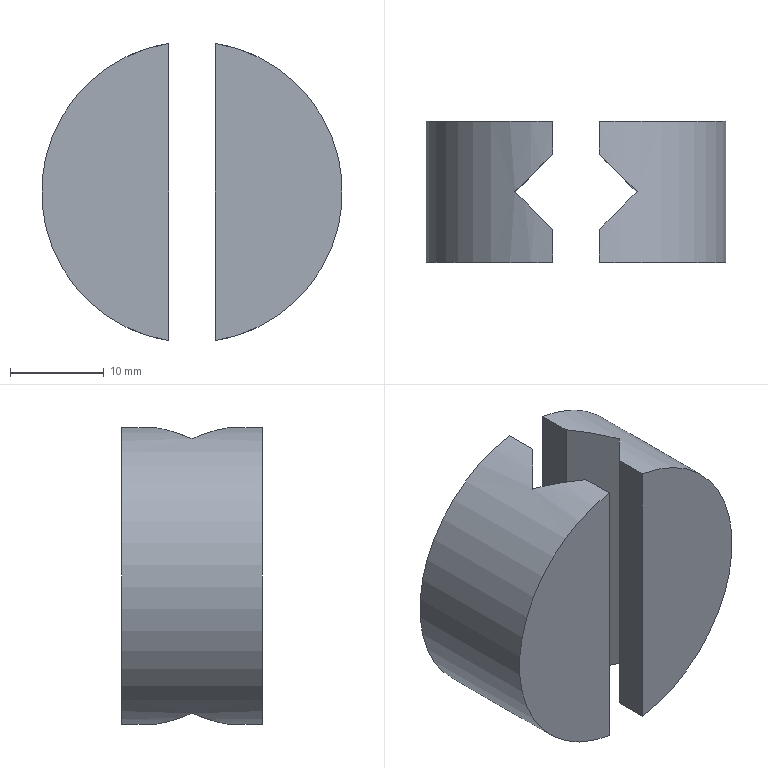Part | STEP file | Shark Fin Adapter | 2 solids | 14 faces | box 32 x 15 x 31.607 mm | volume 8681 mm3 | plane 12 | cylinder 2 | commonest cylinder face diameters 32 x2
STEP:
#1=CARTESIAN_POINT('',(0.,0.,0.));
#2=DIRECTION('',(0.,0.,1.));
#3=DIRECTION('',(1.,0.,0.));
#4=AXIS2_PLACEMENT_3D('',#1,#2,#3);
#5=CARTESIAN_POINT('',(2.5,7.5,15.803));
#6=VERTEX_POINT('',#5);
#7=CARTESIAN_POINT('',(2.5,7.5,-15.803));
#8=VERTEX_POINT('',#7);
#9=CARTESIAN_POINT('',(0.,7.5,0.));
#10=DIRECTION('',(0.,1.,0.));
#11=DIRECTION('',(0.,0.,1.));
#12=AXIS2_PLACEMENT_3D('',#9,#10,#11);
#13=CIRCLE('',#12,16.);
#14=CARTESIAN_POINT('',(0.,7.5,0.));
#15=DIRECTION('',(0.,-1.,0.));
#16=DIRECTION('',(0.,0.,-1.));
#17=AXIS2_PLACEMENT_3D('',#14,#15,#16);
#18=CYLINDRICAL_SURFACE('',#17,16.);
#19=CARTESIAN_POINT('',(3.142,0.));
#20=DIRECTION('',(-1.,0.));
#21=VECTOR('',#20,1.);
#22=LINE('',#19,#21);
#23=(GEOMETRIC_REPRESENTATION_CONTEXT(2)PARAMETRIC_REPRESENTATION_CONTEXT()REPRESENTATION_CONTEXT('',''));
#24=DEFINITIONAL_REPRESENTATION('',(#22),#23);
#25=PCURVE('',#18,#24);
#26=CARTESIAN_POINT('',(0.,7.5,0.));
#27=DIRECTION('',(0.,1.,0.));
#28=DIRECTION('',(0.,0.,1.));
#29=AXIS2_PLACEMENT_3D('',#26,#27,#28);
#30=PLANE('',#29);
#31=CARTESIAN_POINT('',(0.,0.));
#32=DIRECTION('',(1.,0.));
#33=AXIS2_PLACEMENT_2D('',#31,#32);
#34=CIRCLE('',#33,16.);
#35=(GEOMETRIC_REPRESENTATION_CONTEXT(2)PARAMETRIC_REPRESENTATION_CONTEXT()REPRESENTATION_CONTEXT('',''));
#36=DEFINITIONAL_REPRESENTATION('',(#34),#35);
#37=PCURVE('',#30,#36);
#38=SURFACE_CURVE('',#13,(#25,#37),.PCURVE_S1.);
#39=EDGE_CURVE('',#6,#8,#38,.T.);
#40=ORIENTED_EDGE('',*,*,#39,.F.);
#41=CARTESIAN_POINT('',(2.5,4.,15.803));
#42=VERTEX_POINT('',#41);
#43=CARTESIAN_POINT('',(2.5,7.5,15.803));
#44=DIRECTION('',(0.,-1.,0.));
#45=VECTOR('',#44,1.);
#46=LINE('',#43,#45);
#47=CARTESIAN_POINT('',(2.985,0.));
#48=DIRECTION('',(0.,1.));
#49=VECTOR('',#48,1.);
#50=LINE('',#47,#49);
#51=(GEOMETRIC_REPRESENTATION_CONTEXT(2)PARAMETRIC_REPRESENTATION_CONTEXT()REPRESENTATION_CONTEXT('',''));
#52=DEFINITIONAL_REPRESENTATION('',(#50),#51);
#53=PCURVE('',#18,#52);
#54=CARTESIAN_POINT('',(2.5,4.,-25.));
#55=DIRECTION('',(1.,0.,0.));
#56=DIRECTION('',(0.,1.,0.));
#57=AXIS2_PLACEMENT_3D('',#54,#55,#56);
#58=PLANE('',#57);
#59=CARTESIAN_POINT('',(3.5,40.803));
#60=DIRECTION('',(-1.,0.));
#61=VECTOR('',#60,1.);
#62=LINE('',#59,#61);
#63=(GEOMETRIC_REPRESENTATION_CONTEXT(2)PARAMETRIC_REPRESENTATION_CONTEXT()REPRESENTATION_CONTEXT('',''));
#64=DEFINITIONAL_REPRESENTATION('',(#62),#63);
#65=PCURVE('',#58,#64);
#66=SURFACE_CURVE('',#46,(#53,#65),.PCURVE_S1.);
#67=EDGE_CURVE('',#6,#42,#66,.T.);
#68=ORIENTED_EDGE('',*,*,#67,.T.);
#69=CARTESIAN_POINT('',(6.5,0.,14.62));
#70=VERTEX_POINT('',#69);
#71=CARTESIAN_POINT('',(2.5,4.,15.803));
#72=CARTESIAN_POINT('',(3.881,2.619,15.585));
#73=CARTESIAN_POINT('',(5.222,1.278,15.188));
#74=CARTESIAN_POINT('',(6.5,0.,14.62));
#75=(BOUNDED_CURVE()B_SPLINE_CURVE(3,(#71,#72,#73,#74),.UNSPECIFIED.,.F.,.F.)B_SPLINE_CURVE_WITH_KNOTS((4,4),(4.869,5.131),.PIECEWISE_BEZIER_KNOTS.)CURVE()GEOMETRIC_REPRESENTATION_ITEM()RATIONAL_B_SPLINE_CURVE((1.,0.9943,0.9943,1.))REPRESENTATION_ITEM(''));
#76=CARTESIAN_POINT('',(2.985,3.5));
#77=CARTESIAN_POINT('',(2.981,3.562));
#78=CARTESIAN_POINT('',(2.973,3.687));
#79=CARTESIAN_POINT('',(2.961,3.874));
#80=CARTESIAN_POINT('',(2.949,4.061));
#81=CARTESIAN_POINT('',(2.937,4.247));
#82=CARTESIAN_POINT('',(2.925,4.433));
#83=CARTESIAN_POINT('',(2.913,4.619));
#84=CARTESIAN_POINT('',(2.902,4.804));
#85=CARTESIAN_POINT('',(2.89,4.988));
#86=CARTESIAN_POINT('',(2.878,5.172));
#87=CARTESIAN_POINT('',(2.866,5.356));
#88=CARTESIAN_POINT('',(2.854,5.539));
#89=CARTESIAN_POINT('',(2.842,5.721));
#90=CARTESIAN_POINT('',(2.83,5.903));
#91=CARTESIAN_POINT('',(2.818,6.084));
#92=CARTESIAN_POINT('',(2.806,6.264));
#93=CARTESIAN_POINT('',(2.794,6.443));
#94=CARTESIAN_POINT('',(2.783,6.622));
#95=CARTESIAN_POINT('',(2.771,6.799));
#96=CARTESIAN_POINT('',(2.759,6.976));
#97=CARTESIAN_POINT('',(2.747,7.152));
#98=CARTESIAN_POINT('',(2.735,7.326));
#99=CARTESIAN_POINT('',(2.727,7.442));
#100=CARTESIAN_POINT('',(2.723,7.5));
#101=B_SPLINE_CURVE_WITH_KNOTS('',3,(#76,#77,#78,#79,#80,#81,#82,#83,#84,#85,#86,#87,#88,#89,#90,#91,#92,#93,#94,#95,#96,#97,#98,#99,#100),.UNSPECIFIED.,.F.,.F.,(4,1,1,1,1,1,1,1,1,1,1,1,1,1,1,1,1,1,1,1,1,1,4),(4.869,4.881,4.893,4.905,4.917,4.929,4.941,4.952,4.964,4.976,4.988,5.,5.012,5.024,5.036,5.048,5.059,5.071,5.083,5.095,5.107,5.119,5.131),.QUASI_UNIFORM_KNOTS.);
#102=(GEOMETRIC_REPRESENTATION_CONTEXT(2)PARAMETRIC_REPRESENTATION_CONTEXT()REPRESENTATION_CONTEXT('',''));
#103=DEFINITIONAL_REPRESENTATION('',(#101),#102);
#104=PCURVE('',#18,#103);
#105=CARTESIAN_POINT('',(6.5,0.,-25.));
#106=DIRECTION('',(0.7071,0.7071,0.));
#107=DIRECTION('',(-0.7071,0.7071,0.));
#108=AXIS2_PLACEMENT_3D('',#105,#106,#107);
#109=PLANE('',#108);
#110=CARTESIAN_POINT('',(5.657,40.803));
#111=CARTESIAN_POINT('',(3.704,40.585));
#112=CARTESIAN_POINT('',(1.807,40.188));
#113=CARTESIAN_POINT('',(0.,39.62));
#114=(BOUNDED_CURVE()B_SPLINE_CURVE(3,(#110,#111,#112,#113),.UNSPECIFIED.,.F.,.F.)B_SPLINE_CURVE_WITH_KNOTS((4,4),(4.869,5.131),.PIECEWISE_BEZIER_KNOTS.)CURVE()GEOMETRIC_REPRESENTATION_ITEM()RATIONAL_B_SPLINE_CURVE((1.,0.9943,0.9943,1.))REPRESENTATION_ITEM(''));
#115=(GEOMETRIC_REPRESENTATION_CONTEXT(2)PARAMETRIC_REPRESENTATION_CONTEXT()REPRESENTATION_CONTEXT('',''));
#116=DEFINITIONAL_REPRESENTATION('',(#114),#115);
#117=PCURVE('',#109,#116);
#118=SURFACE_CURVE('',#75,(#104,#117),.PCURVE_S1.);
#119=EDGE_CURVE('',#42,#70,#118,.T.);
#120=ORIENTED_EDGE('',*,*,#119,.T.);
#121=CARTESIAN_POINT('',(2.5,-4.,15.803));
#122=VERTEX_POINT('',#121);
#123=CARTESIAN_POINT('',(6.5,0.,14.62));
#124=CARTESIAN_POINT('',(5.222,-1.278,15.188));
#125=CARTESIAN_POINT('',(3.881,-2.619,15.585));
#126=CARTESIAN_POINT('',(2.5,-4.,15.803));
#127=(BOUNDED_CURVE()B_SPLINE_CURVE(3,(#123,#124,#125,#126),.UNSPECIFIED.,.F.,.F.)B_SPLINE_CURVE_WITH_KNOTS((4,4),(4.294,4.555),.PIECEWISE_BEZIER_KNOTS.)CURVE()GEOMETRIC_REPRESENTATION_ITEM()RATIONAL_B_SPLINE_CURVE((1.,0.9943,0.9943,1.))REPRESENTATION_ITEM(''));
#128=CARTESIAN_POINT('',(2.723,7.5));
#129=CARTESIAN_POINT('',(2.727,7.558));
#130=CARTESIAN_POINT('',(2.735,7.674));
#131=CARTESIAN_POINT('',(2.747,7.848));
#132=CARTESIAN_POINT('',(2.759,8.024));
#133=CARTESIAN_POINT('',(2.771,8.201));
#134=CARTESIAN_POINT('',(2.783,8.378));
#135=CARTESIAN_POINT('',(2.794,8.557));
#136=CARTESIAN_POINT('',(2.806,8.736));
#137=CARTESIAN_POINT('',(2.818,8.916));
#138=CARTESIAN_POINT('',(2.83,9.097));
#139=CARTESIAN_POINT('',(2.842,9.279));
#140=CARTESIAN_POINT('',(2.854,9.461));
#141=CARTESIAN_POINT('',(2.866,9.644));
#142=CARTESIAN_POINT('',(2.878,9.828));
#143=CARTESIAN_POINT('',(2.89,10.012));
#144=CARTESIAN_POINT('',(2.902,10.196));
#145=CARTESIAN_POINT('',(2.913,10.381));
#146=CARTESIAN_POINT('',(2.925,10.567));
#147=CARTESIAN_POINT('',(2.937,10.753));
#148=CARTESIAN_POINT('',(2.949,10.939));
#149=CARTESIAN_POINT('',(2.961,11.126));
#150=CARTESIAN_POINT('',(2.973,11.313));
#151=CARTESIAN_POINT('',(2.981,11.438));
#152=CARTESIAN_POINT('',(2.985,11.5));
#153=B_SPLINE_CURVE_WITH_KNOTS('',3,(#128,#129,#130,#131,#132,#133,#134,#135,#136,#137,#138,#139,#140,#141,#142,#143,#144,#145,#146,#147,#148,#149,#150,#151,#152),.UNSPECIFIED.,.F.,.F.,(4,1,1,1,1,1,1,1,1,1,1,1,1,1,1,1,1,1,1,1,1,1,4),(4.294,4.306,4.318,4.33,4.342,4.353,4.365,4.377,4.389,4.401,4.413,4.425,4.437,4.449,4.46,4.472,4.484,4.496,4.508,4.52,4.532,4.544,4.555),.QUASI_UNIFORM_KNOTS.);
#154=(GEOMETRIC_REPRESENTATION_CONTEXT(2)PARAMETRIC_REPRESENTATION_CONTEXT()REPRESENTATION_CONTEXT('',''));
#155=DEFINITIONAL_REPRESENTATION('',(#153),#154);
#156=PCURVE('',#18,#155);
#157=CARTESIAN_POINT('',(6.5,0.,-25.));
#158=DIRECTION('',(0.7071,-0.7071,0.));
#159=DIRECTION('',(0.7071,0.7071,0.));
#160=AXIS2_PLACEMENT_3D('',#157,#158,#159);
#161=PLANE('',#160);
#162=CARTESIAN_POINT('',(0.,39.62));
#163=CARTESIAN_POINT('',(-1.807,40.188));
#164=CARTESIAN_POINT('',(-3.704,40.585));
#165=CARTESIAN_POINT('',(-5.657,40.803));
#166=(BOUNDED_CURVE()B_SPLINE_CURVE(3,(#162,#163,#164,#165),.UNSPECIFIED.,.F.,.F.)B_SPLINE_CURVE_WITH_KNOTS((4,4),(4.294,4.555),.PIECEWISE_BEZIER_KNOTS.)CURVE()GEOMETRIC_REPRESENTATION_ITEM()RATIONAL_B_SPLINE_CURVE((1.,0.9943,0.9943,1.))REPRESENTATION_ITEM(''));
#167=(GEOMETRIC_REPRESENTATION_CONTEXT(2)PARAMETRIC_REPRESENTATION_CONTEXT()REPRESENTATION_CONTEXT('',''));
#168=DEFINITIONAL_REPRESENTATION('',(#166),#167);
#169=PCURVE('',#161,#168);
#170=SURFACE_CURVE('',#127,(#156,#169),.PCURVE_S1.);
#171=EDGE_CURVE('',#70,#122,#170,.T.);
#172=ORIENTED_EDGE('',*,*,#171,.T.);
#173=CARTESIAN_POINT('',(2.5,-7.5,15.803));
#174=VERTEX_POINT('',#173);
#175=CARTESIAN_POINT('',(2.5,7.5,15.803));
#176=DIRECTION('',(0.,-1.,0.));
#177=VECTOR('',#176,1.);
#178=LINE('',#175,#177);
#179=CARTESIAN_POINT('',(2.985,0.));
#180=DIRECTION('',(0.,1.));
#181=VECTOR('',#180,1.);
#182=LINE('',#179,#181);
#183=(GEOMETRIC_REPRESENTATION_CONTEXT(2)PARAMETRIC_REPRESENTATION_CONTEXT()REPRESENTATION_CONTEXT('',''));
#184=DEFINITIONAL_REPRESENTATION('',(#182),#183);
#185=PCURVE('',#18,#184);
#186=CARTESIAN_POINT('',(2.5,-4.,-25.));
#187=DIRECTION('',(1.,0.,0.));
#188=DIRECTION('',(0.,1.,0.));
#189=AXIS2_PLACEMENT_3D('',#186,#187,#188);
#190=PLANE('',#189);
#191=CARTESIAN_POINT('',(11.5,40.803));
#192=DIRECTION('',(-1.,0.));
#193=VECTOR('',#192,1.);
#194=LINE('',#191,#193);
#195=(GEOMETRIC_REPRESENTATION_CONTEXT(2)PARAMETRIC_REPRESENTATION_CONTEXT()REPRESENTATION_CONTEXT('',''));
#196=DEFINITIONAL_REPRESENTATION('',(#194),#195);
#197=PCURVE('',#190,#196);
#198=SURFACE_CURVE('',#178,(#185,#197),.PCURVE_S1.);
#199=EDGE_CURVE('',#122,#174,#198,.T.);
#200=ORIENTED_EDGE('',*,*,#199,.T.);
#201=CARTESIAN_POINT('',(2.5,-7.5,-15.803));
#202=VERTEX_POINT('',#201);
#203=CARTESIAN_POINT('',(0.,-7.5,0.));
#204=DIRECTION('',(0.,1.,0.));
#205=DIRECTION('',(0.,0.,1.));
#206=AXIS2_PLACEMENT_3D('',#203,#204,#205);
#207=CIRCLE('',#206,16.);
#208=CARTESIAN_POINT('',(3.142,15.));
#209=DIRECTION('',(-1.,0.));
#210=VECTOR('',#209,1.);
#211=LINE('',#208,#210);
#212=(GEOMETRIC_REPRESENTATION_CONTEXT(2)PARAMETRIC_REPRESENTATION_CONTEXT()REPRESENTATION_CONTEXT('',''));
#213=DEFINITIONAL_REPRESENTATION('',(#211),#212);
#214=PCURVE('',#18,#213);
#215=CARTESIAN_POINT('',(0.,-7.5,0.));
#216=DIRECTION('',(0.,1.,0.));
#217=DIRECTION('',(0.,0.,1.));
#218=AXIS2_PLACEMENT_3D('',#215,#216,#217);
#219=PLANE('',#218);
#220=CARTESIAN_POINT('',(0.,0.));
#221=DIRECTION('',(1.,0.));
#222=AXIS2_PLACEMENT_2D('',#220,#221);
#223=CIRCLE('',#222,16.);
#224=(GEOMETRIC_REPRESENTATION_CONTEXT(2)PARAMETRIC_REPRESENTATION_CONTEXT()REPRESENTATION_CONTEXT('',''));
#225=DEFINITIONAL_REPRESENTATION('',(#223),#224);
#226=PCURVE('',#219,#225);
#227=SURFACE_CURVE('',#207,(#214,#226),.PCURVE_S1.);
#228=EDGE_CURVE('',#174,#202,#227,.T.);
#229=ORIENTED_EDGE('',*,*,#228,.T.);
#230=CARTESIAN_POINT('',(2.5,-4.,-15.803));
#231=VERTEX_POINT('',#230);
#232=CARTESIAN_POINT('',(2.5,7.5,-15.803));
#233=DIRECTION('',(0.,1.,0.));
#234=VECTOR('',#233,1.);
#235=LINE('',#232,#234);
#236=CARTESIAN_POINT('',(0.1569,0.));
#237=DIRECTION('',(0.,-1.));
#238=VECTOR('',#237,1.);
#239=LINE('',#236,#238);
#240=(GEOMETRIC_REPRESENTATION_CONTEXT(2)PARAMETRIC_REPRESENTATION_CONTEXT()REPRESENTATION_CONTEXT('',''));
#241=DEFINITIONAL_REPRESENTATION('',(#239),#240);
#242=PCURVE('',#18,#241);
#243=CARTESIAN_POINT('',(11.5,9.197));
#244=DIRECTION('',(1.,0.));
#245=VECTOR('',#244,1.);
#246=LINE('',#243,#245);
#247=(GEOMETRIC_REPRESENTATION_CONTEXT(2)PARAMETRIC_REPRESENTATION_CONTEXT()REPRESENTATION_CONTEXT('',''));
#248=DEFINITIONAL_REPRESENTATION('',(#246),#247);
#249=PCURVE('',#190,#248);
#250=SURFACE_CURVE('',#235,(#242,#249),.PCURVE_S1.);
#251=EDGE_CURVE('',#202,#231,#250,.T.);
#252=ORIENTED_EDGE('',*,*,#251,.T.);
#253=CARTESIAN_POINT('',(6.5,0.,-14.62));
#254=VERTEX_POINT('',#253);
#255=CARTESIAN_POINT('',(2.5,-4.,-15.803));
#256=CARTESIAN_POINT('',(3.881,-2.619,-15.585));
#257=CARTESIAN_POINT('',(5.222,-1.278,-15.188));
#258=CARTESIAN_POINT('',(6.5,0.,-14.62));
#259=(BOUNDED_CURVE()B_SPLINE_CURVE(3,(#255,#256,#257,#258),.UNSPECIFIED.,.F.,.F.)B_SPLINE_CURVE_WITH_KNOTS((4,4),(1.728,1.989),.PIECEWISE_BEZIER_KNOTS.)CURVE()GEOMETRIC_REPRESENTATION_ITEM()RATIONAL_B_SPLINE_CURVE((1.,0.9943,0.9943,1.))REPRESENTATION_ITEM(''));
#260=CARTESIAN_POINT('',(0.1569,11.5));
#261=CARTESIAN_POINT('',(0.1608,11.438));
#262=CARTESIAN_POINT('',(0.1687,11.313));
#263=CARTESIAN_POINT('',(0.1806,11.126));
#264=CARTESIAN_POINT('',(0.1925,10.939));
#265=CARTESIAN_POINT('',(0.2044,10.753));
#266=CARTESIAN_POINT('',(0.2162,10.567));
#267=CARTESIAN_POINT('',(0.2281,10.381));
#268=CARTESIAN_POINT('',(0.24,10.196));
#269=CARTESIAN_POINT('',(0.2519,10.012));
#270=CARTESIAN_POINT('',(0.2638,9.828));
#271=CARTESIAN_POINT('',(0.2757,9.644));
#272=CARTESIAN_POINT('',(0.2876,9.461));
#273=CARTESIAN_POINT('',(0.2995,9.279));
#274=CARTESIAN_POINT('',(0.3114,9.097));
#275=CARTESIAN_POINT('',(0.3233,8.916));
#276=CARTESIAN_POINT('',(0.3352,8.736));
#277=CARTESIAN_POINT('',(0.3471,8.557));
#278=CARTESIAN_POINT('',(0.359,8.378));
#279=CARTESIAN_POINT('',(0.3709,8.201));
#280=CARTESIAN_POINT('',(0.3828,8.024));
#281=CARTESIAN_POINT('',(0.3946,7.848));
#282=CARTESIAN_POINT('',(0.4065,7.674));
#283=CARTESIAN_POINT('',(0.4144,7.558));
#284=CARTESIAN_POINT('',(0.4183,7.5));
#285=B_SPLINE_CURVE_WITH_KNOTS('',3,(#260,#261,#262,#263,#264,#265,#266,#267,#268,#269,#270,#271,#272,#273,#274,#275,#276,#277,#278,#279,#280,#281,#282,#283,#284),.UNSPECIFIED.,.F.,.F.,(4,1,1,1,1,1,1,1,1,1,1,1,1,1,1,1,1,1,1,1,1,1,4),(1.728,1.74,1.751,1.763,1.775,1.787,1.799,1.811,1.823,1.835,1.847,1.858,1.87,1.882,1.894,1.906,1.918,1.93,1.942,1.953,1.965,1.977,1.989),.QUASI_UNIFORM_KNOTS.);
#286=(GEOMETRIC_REPRESENTATION_CONTEXT(2)PARAMETRIC_REPRESENTATION_CONTEXT()REPRESENTATION_CONTEXT('',''));
#287=DEFINITIONAL_REPRESENTATION('',(#285),#286);
#288=PCURVE('',#18,#287);
#289=CARTESIAN_POINT('',(-5.657,9.197));
#290=CARTESIAN_POINT('',(-3.704,9.415));
#291=CARTESIAN_POINT('',(-1.807,9.812));
#292=CARTESIAN_POINT('',(0.,10.38));
#293=(BOUNDED_CURVE()B_SPLINE_CURVE(3,(#289,#290,#291,#292),.UNSPECIFIED.,.F.,.F.)B_SPLINE_CURVE_WITH_KNOTS((4,4),(1.728,1.989),.PIECEWISE_BEZIER_KNOTS.)CURVE()GEOMETRIC_REPRESENTATION_ITEM()RATIONAL_B_SPLINE_CURVE((1.,0.9943,0.9943,1.))REPRESENTATION_ITEM(''));
#294=(GEOMETRIC_REPRESENTATION_CONTEXT(2)PARAMETRIC_REPRESENTATION_CONTEXT()REPRESENTATION_CONTEXT('',''));
#295=DEFINITIONAL_REPRESENTATION('',(#293),#294);
#296=PCURVE('',#161,#295);
#297=SURFACE_CURVE('',#259,(#288,#296),.PCURVE_S1.);
#298=EDGE_CURVE('',#231,#254,#297,.T.);
#299=ORIENTED_EDGE('',*,*,#298,.T.);
#300=CARTESIAN_POINT('',(2.5,4.,-15.803));
#301=VERTEX_POINT('',#300);
#302=CARTESIAN_POINT('',(6.5,0.,-14.62));
#303=CARTESIAN_POINT('',(5.222,1.278,-15.188));
#304=CARTESIAN_POINT('',(3.881,2.619,-15.585));
#305=CARTESIAN_POINT('',(2.5,4.,-15.803));
#306=(BOUNDED_CURVE()B_SPLINE_CURVE(3,(#302,#303,#304,#305),.UNSPECIFIED.,.F.,.F.)B_SPLINE_CURVE_WITH_KNOTS((4,4),(1.152,1.414),.PIECEWISE_BEZIER_KNOTS.)CURVE()GEOMETRIC_REPRESENTATION_ITEM()RATIONAL_B_SPLINE_CURVE((1.,0.9943,0.9943,1.))REPRESENTATION_ITEM(''));
#307=CARTESIAN_POINT('',(0.4183,7.5));
#308=CARTESIAN_POINT('',(0.4144,7.442));
#309=CARTESIAN_POINT('',(0.4065,7.326));
#310=CARTESIAN_POINT('',(0.3946,7.152));
#311=CARTESIAN_POINT('',(0.3828,6.976));
#312=CARTESIAN_POINT('',(0.3709,6.799));
#313=CARTESIAN_POINT('',(0.359,6.622));
#314=CARTESIAN_POINT('',(0.3471,6.443));
#315=CARTESIAN_POINT('',(0.3352,6.264));
#316=CARTESIAN_POINT('',(0.3233,6.084));
#317=CARTESIAN_POINT('',(0.3114,5.903));
#318=CARTESIAN_POINT('',(0.2995,5.721));
#319=CARTESIAN_POINT('',(0.2876,5.539));
#320=CARTESIAN_POINT('',(0.2757,5.356));
#321=CARTESIAN_POINT('',(0.2638,5.172));
#322=CARTESIAN_POINT('',(0.2519,4.988));
#323=CARTESIAN_POINT('',(0.24,4.804));
#324=CARTESIAN_POINT('',(0.2281,4.619));
#325=CARTESIAN_POINT('',(0.2162,4.433));
#326=CARTESIAN_POINT('',(0.2044,4.247));
#327=CARTESIAN_POINT('',(0.1925,4.061));
#328=CARTESIAN_POINT('',(0.1806,3.874));
#329=CARTESIAN_POINT('',(0.1687,3.687));
#330=CARTESIAN_POINT('',(0.1608,3.562));
#331=CARTESIAN_POINT('',(0.1569,3.5));
#332=B_SPLINE_CURVE_WITH_KNOTS('',3,(#307,#308,#309,#310,#311,#312,#313,#314,#315,#316,#317,#318,#319,#320,#321,#322,#323,#324,#325,#326,#327,#328,#329,#330,#331),.UNSPECIFIED.,.F.,.F.,(4,1,1,1,1,1,1,1,1,1,1,1,1,1,1,1,1,1,1,1,1,1,4),(1.152,1.164,1.176,1.188,1.2,1.212,1.224,1.236,1.248,1.259,1.271,1.283,1.295,1.307,1.319,1.331,1.343,1.354,1.366,1.378,1.39,1.402,1.414),.QUASI_UNIFORM_KNOTS.);
#333=(GEOMETRIC_REPRESENTATION_CONTEXT(2)PARAMETRIC_REPRESENTATION_CONTEXT()REPRESENTATION_CONTEXT('',''));
#334=DEFINITIONAL_REPRESENTATION('',(#332),#333);
#335=PCURVE('',#18,#334);
#336=CARTESIAN_POINT('',(0.,10.38));
#337=CARTESIAN_POINT('',(1.807,9.812));
#338=CARTESIAN_POINT('',(3.704,9.415));
#339=CARTESIAN_POINT('',(5.657,9.197));
#340=(BOUNDED_CURVE()B_SPLINE_CURVE(3,(#336,#337,#338,#339),.UNSPECIFIED.,.F.,.F.)B_SPLINE_CURVE_WITH_KNOTS((4,4),(1.152,1.414),.PIECEWISE_BEZIER_KNOTS.)CURVE()GEOMETRIC_REPRESENTATION_ITEM()RATIONAL_B_SPLINE_CURVE((1.,0.9943,0.9943,1.))REPRESENTATION_ITEM(''));
#341=(GEOMETRIC_REPRESENTATION_CONTEXT(2)PARAMETRIC_REPRESENTATION_CONTEXT()REPRESENTATION_CONTEXT('',''));
#342=DEFINITIONAL_REPRESENTATION('',(#340),#341);
#343=PCURVE('',#109,#342);
#344=SURFACE_CURVE('',#306,(#335,#343),.PCURVE_S1.);
#345=EDGE_CURVE('',#254,#301,#344,.T.);
#346=ORIENTED_EDGE('',*,*,#345,.T.);
#347=CARTESIAN_POINT('',(2.5,7.5,-15.803));
#348=DIRECTION('',(0.,1.,0.));
#349=VECTOR('',#348,1.);
#350=LINE('',#347,#349);
#351=CARTESIAN_POINT('',(0.1569,0.));
#352=DIRECTION('',(0.,-1.));
#353=VECTOR('',#352,1.);
#354=LINE('',#351,#353);
#355=(GEOMETRIC_REPRESENTATION_CONTEXT(2)PARAMETRIC_REPRESENTATION_CONTEXT()REPRESENTATION_CONTEXT('',''));
#356=DEFINITIONAL_REPRESENTATION('',(#354),#355);
#357=PCURVE('',#18,#356);
#358=CARTESIAN_POINT('',(3.5,9.197));
#359=DIRECTION('',(1.,0.));
#360=VECTOR('',#359,1.);
#361=LINE('',#358,#360);
#362=(GEOMETRIC_REPRESENTATION_CONTEXT(2)PARAMETRIC_REPRESENTATION_CONTEXT()REPRESENTATION_CONTEXT('',''));
#363=DEFINITIONAL_REPRESENTATION('',(#361),#362);
#364=PCURVE('',#58,#363);
#365=SURFACE_CURVE('',#350,(#357,#364),.PCURVE_S1.);
#366=EDGE_CURVE('',#301,#8,#365,.T.);
#367=ORIENTED_EDGE('',*,*,#366,.T.);
#368=EDGE_LOOP('',(#40,#68,#120,#172,#200,#229,#252,#299,#346,#367));
#369=FACE_BOUND('',#368,.T.);
#370=ADVANCED_FACE('',(#369),#18,.T.);
#371=ORIENTED_EDGE('',*,*,#228,.F.);
#372=CARTESIAN_POINT('',(2.5,-7.5,0.));
#373=DIRECTION('',(0.,0.,-1.));
#374=VECTOR('',#373,1.);
#375=LINE('',#372,#374);
#376=CARTESIAN_POINT('',(0.,2.5));
#377=DIRECTION('',(-1.,0.));
#378=VECTOR('',#377,1.);
#379=LINE('',#376,#378);
#380=(GEOMETRIC_REPRESENTATION_CONTEXT(2)PARAMETRIC_REPRESENTATION_CONTEXT()REPRESENTATION_CONTEXT('',''));
#381=DEFINITIONAL_REPRESENTATION('',(#379),#380);
#382=PCURVE('',#219,#381);
#383=CARTESIAN_POINT('',(-3.5,25.));
#384=DIRECTION('',(0.,-1.));
#385=VECTOR('',#384,1.);
#386=LINE('',#383,#385);
#387=(GEOMETRIC_REPRESENTATION_CONTEXT(2)PARAMETRIC_REPRESENTATION_CONTEXT()REPRESENTATION_CONTEXT('',''));
#388=DEFINITIONAL_REPRESENTATION('',(#386),#387);
#389=PCURVE('',#190,#388);
#390=SURFACE_CURVE('',#375,(#382,#389),.PCURVE_S1.);
#391=EDGE_CURVE('',#174,#202,#390,.T.);
#392=ORIENTED_EDGE('',*,*,#391,.T.);
#393=EDGE_LOOP('',(#371,#392));
#394=FACE_BOUND('',#393,.T.);
#395=ADVANCED_FACE('',(#394),#219,.F.);
#396=CARTESIAN_POINT('',(2.5,7.5,0.));
#397=DIRECTION('',(0.,0.,-1.));
#398=VECTOR('',#397,1.);
#399=LINE('',#396,#398);
#400=CARTESIAN_POINT('',(0.,2.5));
#401=DIRECTION('',(-1.,0.));
#402=VECTOR('',#401,1.);
#403=LINE('',#400,#402);
#404=(GEOMETRIC_REPRESENTATION_CONTEXT(2)PARAMETRIC_REPRESENTATION_CONTEXT()REPRESENTATION_CONTEXT('',''));
#405=DEFINITIONAL_REPRESENTATION('',(#403),#404);
#406=PCURVE('',#30,#405);
#407=CARTESIAN_POINT('',(3.5,25.));
#408=DIRECTION('',(0.,-1.));
#409=VECTOR('',#408,1.);
#410=LINE('',#407,#409);
#411=(GEOMETRIC_REPRESENTATION_CONTEXT(2)PARAMETRIC_REPRESENTATION_CONTEXT()REPRESENTATION_CONTEXT('',''));
#412=DEFINITIONAL_REPRESENTATION('',(#410),#411);
#413=PCURVE('',#58,#412);
#414=SURFACE_CURVE('',#399,(#406,#413),.PCURVE_S1.);
#415=EDGE_CURVE('',#6,#8,#414,.T.);
#416=ORIENTED_EDGE('',*,*,#415,.F.);
#417=ORIENTED_EDGE('',*,*,#39,.T.);
#418=EDGE_LOOP('',(#416,#417));
#419=FACE_BOUND('',#418,.T.);
#420=ADVANCED_FACE('',(#419),#30,.T.);
#421=CARTESIAN_POINT('',(6.5,0.,-25.));
#422=DIRECTION('',(0.,0.,1.));
#423=VECTOR('',#422,1.);
#424=LINE('',#421,#423);
#425=CARTESIAN_POINT('',(0.,0.));
#426=DIRECTION('',(0.,1.));
#427=VECTOR('',#426,1.);
#428=LINE('',#425,#427);
#429=(GEOMETRIC_REPRESENTATION_CONTEXT(2)PARAMETRIC_REPRESENTATION_CONTEXT()REPRESENTATION_CONTEXT('',''));
#430=DEFINITIONAL_REPRESENTATION('',(#428),#429);
#431=PCURVE('',#109,#430);
#432=CARTESIAN_POINT('',(0.,0.));
#433=DIRECTION('',(0.,1.));
#434=VECTOR('',#433,1.);
#435=LINE('',#432,#434);
#436=(GEOMETRIC_REPRESENTATION_CONTEXT(2)PARAMETRIC_REPRESENTATION_CONTEXT()REPRESENTATION_CONTEXT('',''));
#437=DEFINITIONAL_REPRESENTATION('',(#435),#436);
#438=PCURVE('',#161,#437);
#439=SURFACE_CURVE('',#424,(#431,#438),.PCURVE_S1.);
#440=EDGE_CURVE('',#254,#70,#439,.T.);
#441=ORIENTED_EDGE('',*,*,#440,.T.);
#442=ORIENTED_EDGE('',*,*,#119,.F.);
#443=CARTESIAN_POINT('',(2.5,4.,-25.));
#444=DIRECTION('',(0.,0.,1.));
#445=VECTOR('',#444,1.);
#446=LINE('',#443,#445);
#447=CARTESIAN_POINT('',(5.657,0.));
#448=DIRECTION('',(0.,1.));
#449=VECTOR('',#448,1.);
#450=LINE('',#447,#449);
#451=(GEOMETRIC_REPRESENTATION_CONTEXT(2)PARAMETRIC_REPRESENTATION_CONTEXT()REPRESENTATION_CONTEXT('',''));
#452=DEFINITIONAL_REPRESENTATION('',(#450),#451);
#453=PCURVE('',#109,#452);
#454=CARTESIAN_POINT('',(0.,0.));
#455=DIRECTION('',(0.,1.));
#456=VECTOR('',#455,1.);
#457=LINE('',#454,#456);
#458=(GEOMETRIC_REPRESENTATION_CONTEXT(2)PARAMETRIC_REPRESENTATION_CONTEXT()REPRESENTATION_CONTEXT('',''));
#459=DEFINITIONAL_REPRESENTATION('',(#457),#458);
#460=PCURVE('',#58,#459);
#461=SURFACE_CURVE('',#446,(#453,#460),.PCURVE_S1.);
#462=EDGE_CURVE('',#301,#42,#461,.T.);
#463=ORIENTED_EDGE('',*,*,#462,.F.);
#464=ORIENTED_EDGE('',*,*,#345,.F.);
#465=EDGE_LOOP('',(#441,#442,#463,#464));
#466=FACE_BOUND('',#465,.T.);
#467=ADVANCED_FACE('',(#466),#109,.F.);
#468=CARTESIAN_POINT('',(2.5,-4.,-25.));
#469=DIRECTION('',(0.,0.,1.));
#470=VECTOR('',#469,1.);
#471=LINE('',#468,#470);
#472=CARTESIAN_POINT('',(-5.657,0.));
#473=DIRECTION('',(0.,1.));
#474=VECTOR('',#473,1.);
#475=LINE('',#472,#474);
#476=(GEOMETRIC_REPRESENTATION_CONTEXT(2)PARAMETRIC_REPRESENTATION_CONTEXT()REPRESENTATION_CONTEXT('',''));
#477=DEFINITIONAL_REPRESENTATION('',(#475),#476);
#478=PCURVE('',#161,#477);
#479=CARTESIAN_POINT('',(0.,0.));
#480=DIRECTION('',(0.,1.));
#481=VECTOR('',#480,1.);
#482=LINE('',#479,#481);
#483=(GEOMETRIC_REPRESENTATION_CONTEXT(2)PARAMETRIC_REPRESENTATION_CONTEXT()REPRESENTATION_CONTEXT('',''));
#484=DEFINITIONAL_REPRESENTATION('',(#482),#483);
#485=PCURVE('',#190,#484);
#486=SURFACE_CURVE('',#471,(#478,#485),.PCURVE_S1.);
#487=EDGE_CURVE('',#231,#122,#486,.T.);
#488=ORIENTED_EDGE('',*,*,#487,.T.);
#489=ORIENTED_EDGE('',*,*,#171,.F.);
#490=ORIENTED_EDGE('',*,*,#440,.F.);
#491=ORIENTED_EDGE('',*,*,#298,.F.);
#492=EDGE_LOOP('',(#488,#489,#490,#491));
#493=FACE_BOUND('',#492,.T.);
#494=ADVANCED_FACE('',(#493),#161,.F.);
#495=ORIENTED_EDGE('',*,*,#415,.T.);
#496=ORIENTED_EDGE('',*,*,#366,.F.);
#497=ORIENTED_EDGE('',*,*,#462,.T.);
#498=ORIENTED_EDGE('',*,*,#67,.F.);
#499=EDGE_LOOP('',(#495,#496,#497,#498));
#500=FACE_BOUND('',#499,.T.);
#501=ADVANCED_FACE('',(#500),#58,.F.);
#502=ORIENTED_EDGE('',*,*,#487,.F.);
#503=ORIENTED_EDGE('',*,*,#251,.F.);
#504=ORIENTED_EDGE('',*,*,#391,.F.);
#505=ORIENTED_EDGE('',*,*,#199,.F.);
#506=EDGE_LOOP('',(#502,#503,#504,#505));
#507=FACE_BOUND('',#506,.T.);
#508=ADVANCED_FACE('',(#507),#190,.F.);
#509=CLOSED_SHELL('',(#370,#395,#420,#467,#494,#501,#508));
#510=MANIFOLD_SOLID_BREP('',#509);
#511=CARTESIAN_POINT('',(-2.5,-7.5,-15.803));
#512=VERTEX_POINT('',#511);
#513=CARTESIAN_POINT('',(-2.5,-7.5,15.803));
#514=VERTEX_POINT('',#513);
#515=CARTESIAN_POINT('',(0.,-7.5,0.));
#516=DIRECTION('',(0.,1.,0.));
#517=DIRECTION('',(0.,0.,1.));
#518=AXIS2_PLACEMENT_3D('',#515,#516,#517);
#519=CIRCLE('',#518,16.);
#520=CARTESIAN_POINT('',(0.,-7.5,0.));
#521=DIRECTION('',(0.,1.,0.));
#522=DIRECTION('',(0.,0.,1.));
#523=AXIS2_PLACEMENT_3D('',#520,#521,#522);
#524=PLANE('',#523);
#525=CARTESIAN_POINT('',(0.,0.));
#526=DIRECTION('',(1.,0.));
#527=AXIS2_PLACEMENT_2D('',#525,#526);
#528=CIRCLE('',#527,16.);
#529=(GEOMETRIC_REPRESENTATION_CONTEXT(2)PARAMETRIC_REPRESENTATION_CONTEXT()REPRESENTATION_CONTEXT('',''));
#530=DEFINITIONAL_REPRESENTATION('',(#528),#529);
#531=PCURVE('',#524,#530);
#532=CARTESIAN_POINT('',(0.,7.5,0.));
#533=DIRECTION('',(0.,-1.,0.));
#534=DIRECTION('',(0.,0.,-1.));
#535=AXIS2_PLACEMENT_3D('',#532,#533,#534);
#536=CYLINDRICAL_SURFACE('',#535,16.);
#537=CARTESIAN_POINT('',(9.425,15.));
#538=DIRECTION('',(-1.,0.));
#539=VECTOR('',#538,1.);
#540=LINE('',#537,#539);
#541=(GEOMETRIC_REPRESENTATION_CONTEXT(2)PARAMETRIC_REPRESENTATION_CONTEXT()REPRESENTATION_CONTEXT('',''));
#542=DEFINITIONAL_REPRESENTATION('',(#540),#541);
#543=PCURVE('',#536,#542);
#544=SURFACE_CURVE('',#519,(#531,#543),.PCURVE_S1.);
#545=EDGE_CURVE('',#512,#514,#544,.T.);
#546=ORIENTED_EDGE('',*,*,#545,.F.);
#547=CARTESIAN_POINT('',(-2.5,-7.5,0.));
#548=DIRECTION('',(0.,0.,1.));
#549=VECTOR('',#548,1.);
#550=LINE('',#547,#549);
#551=CARTESIAN_POINT('',(0.,-2.5));
#552=DIRECTION('',(1.,0.));
#553=VECTOR('',#552,1.);
#554=LINE('',#551,#553);
#555=(GEOMETRIC_REPRESENTATION_CONTEXT(2)PARAMETRIC_REPRESENTATION_CONTEXT()REPRESENTATION_CONTEXT('',''));
#556=DEFINITIONAL_REPRESENTATION('',(#554),#555);
#557=PCURVE('',#524,#556);
#558=CARTESIAN_POINT('',(-2.5,-4.,-25.));
#559=DIRECTION('',(-1.,0.,0.));
#560=DIRECTION('',(0.,0.,1.));
#561=AXIS2_PLACEMENT_3D('',#558,#559,#560);
#562=PLANE('',#561);
#563=CARTESIAN_POINT('',(25.,-3.5));
#564=DIRECTION('',(1.,0.));
#565=VECTOR('',#564,1.);
#566=LINE('',#563,#565);
#567=(GEOMETRIC_REPRESENTATION_CONTEXT(2)PARAMETRIC_REPRESENTATION_CONTEXT()REPRESENTATION_CONTEXT('',''));
#568=DEFINITIONAL_REPRESENTATION('',(#566),#567);
#569=PCURVE('',#562,#568);
#570=SURFACE_CURVE('',#550,(#557,#569),.PCURVE_S1.);
#571=EDGE_CURVE('',#512,#514,#570,.T.);
#572=ORIENTED_EDGE('',*,*,#571,.T.);
#573=EDGE_LOOP('',(#546,#572));
#574=FACE_BOUND('',#573,.T.);
#575=ADVANCED_FACE('',(#574),#524,.F.);
#576=CARTESIAN_POINT('',(-2.5,7.5,-15.803));
#577=VERTEX_POINT('',#576);
#578=CARTESIAN_POINT('',(-2.5,7.5,15.803));
#579=VERTEX_POINT('',#578);
#580=CARTESIAN_POINT('',(-2.5,7.5,0.));
#581=DIRECTION('',(0.,0.,1.));
#582=VECTOR('',#581,1.);
#583=LINE('',#580,#582);
#584=CARTESIAN_POINT('',(0.,7.5,0.));
#585=DIRECTION('',(0.,1.,0.));
#586=DIRECTION('',(0.,0.,1.));
#587=AXIS2_PLACEMENT_3D('',#584,#585,#586);
#588=PLANE('',#587);
#589=CARTESIAN_POINT('',(0.,-2.5));
#590=DIRECTION('',(1.,0.));
#591=VECTOR('',#590,1.);
#592=LINE('',#589,#591);
#593=(GEOMETRIC_REPRESENTATION_CONTEXT(2)PARAMETRIC_REPRESENTATION_CONTEXT()REPRESENTATION_CONTEXT('',''));
#594=DEFINITIONAL_REPRESENTATION('',(#592),#593);
#595=PCURVE('',#588,#594);
#596=CARTESIAN_POINT('',(-2.5,4.,-25.));
#597=DIRECTION('',(-1.,0.,0.));
#598=DIRECTION('',(0.,0.,1.));
#599=AXIS2_PLACEMENT_3D('',#596,#597,#598);
#600=PLANE('',#599);
#601=CARTESIAN_POINT('',(25.,3.5));
#602=DIRECTION('',(1.,0.));
#603=VECTOR('',#602,1.);
#604=LINE('',#601,#603);
#605=(GEOMETRIC_REPRESENTATION_CONTEXT(2)PARAMETRIC_REPRESENTATION_CONTEXT()REPRESENTATION_CONTEXT('',''));
#606=DEFINITIONAL_REPRESENTATION('',(#604),#605);
#607=PCURVE('',#600,#606);
#608=SURFACE_CURVE('',#583,(#595,#607),.PCURVE_S1.);
#609=EDGE_CURVE('',#577,#579,#608,.T.);
#610=ORIENTED_EDGE('',*,*,#609,.F.);
#611=CARTESIAN_POINT('',(0.,7.5,0.));
#612=DIRECTION('',(0.,1.,0.));
#613=DIRECTION('',(0.,0.,1.));
#614=AXIS2_PLACEMENT_3D('',#611,#612,#613);
#615=CIRCLE('',#614,16.);
#616=CARTESIAN_POINT('',(0.,0.));
#617=DIRECTION('',(1.,0.));
#618=AXIS2_PLACEMENT_2D('',#616,#617);
#619=CIRCLE('',#618,16.);
#620=(GEOMETRIC_REPRESENTATION_CONTEXT(2)PARAMETRIC_REPRESENTATION_CONTEXT()REPRESENTATION_CONTEXT('',''));
#621=DEFINITIONAL_REPRESENTATION('',(#619),#620);
#622=PCURVE('',#588,#621);
#623=CARTESIAN_POINT('',(9.425,0.));
#624=DIRECTION('',(-1.,0.));
#625=VECTOR('',#624,1.);
#626=LINE('',#623,#625);
#627=(GEOMETRIC_REPRESENTATION_CONTEXT(2)PARAMETRIC_REPRESENTATION_CONTEXT()REPRESENTATION_CONTEXT('',''));
#628=DEFINITIONAL_REPRESENTATION('',(#626),#627);
#629=PCURVE('',#536,#628);
#630=SURFACE_CURVE('',#615,(#622,#629),.PCURVE_S1.);
#631=EDGE_CURVE('',#577,#579,#630,.T.);
#632=ORIENTED_EDGE('',*,*,#631,.T.);
#633=EDGE_LOOP('',(#610,#632));
#634=FACE_BOUND('',#633,.T.);
#635=ADVANCED_FACE('',(#634),#588,.T.);
#636=ORIENTED_EDGE('',*,*,#631,.F.);
#637=CARTESIAN_POINT('',(-2.5,4.,-15.803));
#638=VERTEX_POINT('',#637);
#639=CARTESIAN_POINT('',(-2.5,7.5,-15.803));
#640=DIRECTION('',(0.,-1.,0.));
#641=VECTOR('',#640,1.);
#642=LINE('',#639,#641);
#643=CARTESIAN_POINT('',(6.126,0.));
#644=DIRECTION('',(0.,1.));
#645=VECTOR('',#644,1.);
#646=LINE('',#643,#645);
#647=(GEOMETRIC_REPRESENTATION_CONTEXT(2)PARAMETRIC_REPRESENTATION_CONTEXT()REPRESENTATION_CONTEXT('',''));
#648=DEFINITIONAL_REPRESENTATION('',(#646),#647);
#649=PCURVE('',#536,#648);
#650=CARTESIAN_POINT('',(9.197,3.5));
#651=DIRECTION('',(0.,-1.));
#652=VECTOR('',#651,1.);
#653=LINE('',#650,#652);
#654=(GEOMETRIC_REPRESENTATION_CONTEXT(2)PARAMETRIC_REPRESENTATION_CONTEXT()REPRESENTATION_CONTEXT('',''));
#655=DEFINITIONAL_REPRESENTATION('',(#653),#654);
#656=PCURVE('',#600,#655);
#657=SURFACE_CURVE('',#642,(#649,#656),.PCURVE_S1.);
#658=EDGE_CURVE('',#577,#638,#657,.T.);
#659=ORIENTED_EDGE('',*,*,#658,.T.);
#660=CARTESIAN_POINT('',(-6.5,0.,-14.62));
#661=VERTEX_POINT('',#660);
#662=CARTESIAN_POINT('',(-2.5,4.,-15.803));
#663=CARTESIAN_POINT('',(-3.881,2.619,-15.585));
#664=CARTESIAN_POINT('',(-5.222,1.278,-15.188));
#665=CARTESIAN_POINT('',(-6.5,0.,-14.62));
#666=(BOUNDED_CURVE()B_SPLINE_CURVE(3,(#662,#663,#664,#665),.UNSPECIFIED.,.F.,.F.)B_SPLINE_CURVE_WITH_KNOTS((4,4),(4.869,5.131),.PIECEWISE_BEZIER_KNOTS.)CURVE()GEOMETRIC_REPRESENTATION_ITEM()RATIONAL_B_SPLINE_CURVE((1.,0.9943,0.9943,1.))REPRESENTATION_ITEM(''));
#667=CARTESIAN_POINT('',(6.126,3.5));
#668=CARTESIAN_POINT('',(6.122,3.562));
#669=CARTESIAN_POINT('',(6.114,3.687));
#670=CARTESIAN_POINT('',(6.103,3.874));
#671=CARTESIAN_POINT('',(6.091,4.061));
#672=CARTESIAN_POINT('',(6.079,4.247));
#673=CARTESIAN_POINT('',(6.067,4.433));
#674=CARTESIAN_POINT('',(6.055,4.619));
#675=CARTESIAN_POINT('',(6.043,4.804));
#676=CARTESIAN_POINT('',(6.031,4.988));
#677=CARTESIAN_POINT('',(6.019,5.172));
#678=CARTESIAN_POINT('',(6.007,5.356));
#679=CARTESIAN_POINT('',(5.996,5.539));
#680=CARTESIAN_POINT('',(5.984,5.721));
#681=CARTESIAN_POINT('',(5.972,5.903));
#682=CARTESIAN_POINT('',(5.96,6.084));
#683=CARTESIAN_POINT('',(5.948,6.264));
#684=CARTESIAN_POINT('',(5.936,6.443));
#685=CARTESIAN_POINT('',(5.924,6.622));
#686=CARTESIAN_POINT('',(5.912,6.799));
#687=CARTESIAN_POINT('',(5.9,6.976));
#688=CARTESIAN_POINT('',(5.889,7.152));
#689=CARTESIAN_POINT('',(5.877,7.326));
#690=CARTESIAN_POINT('',(5.869,7.442));
#691=CARTESIAN_POINT('',(5.865,7.5));
#692=B_SPLINE_CURVE_WITH_KNOTS('',3,(#667,#668,#669,#670,#671,#672,#673,#674,#675,#676,#677,#678,#679,#680,#681,#682,#683,#684,#685,#686,#687,#688,#689,#690,#691),.UNSPECIFIED.,.F.,.F.,(4,1,1,1,1,1,1,1,1,1,1,1,1,1,1,1,1,1,1,1,1,1,4),(4.869,4.881,4.893,4.905,4.917,4.929,4.941,4.952,4.964,4.976,4.988,5.,5.012,5.024,5.036,5.048,5.059,5.071,5.083,5.095,5.107,5.119,5.131),.QUASI_UNIFORM_KNOTS.);
#693=(GEOMETRIC_REPRESENTATION_CONTEXT(2)PARAMETRIC_REPRESENTATION_CONTEXT()REPRESENTATION_CONTEXT('',''));
#694=DEFINITIONAL_REPRESENTATION('',(#692),#693);
#695=PCURVE('',#536,#694);
#696=CARTESIAN_POINT('',(-6.5,0.,-25.));
#697=DIRECTION('',(-0.7071,0.7071,0.));
#698=DIRECTION('',(-0.7071,-0.7071,0.));
#699=AXIS2_PLACEMENT_3D('',#696,#697,#698);
#700=PLANE('',#699);
#701=CARTESIAN_POINT('',(-5.657,9.197));
#702=CARTESIAN_POINT('',(-3.704,9.415));
#703=CARTESIAN_POINT('',(-1.807,9.812));
#704=CARTESIAN_POINT('',(0.,10.38));
#705=(BOUNDED_CURVE()B_SPLINE_CURVE(3,(#701,#702,#703,#704),.UNSPECIFIED.,.F.,.F.)B_SPLINE_CURVE_WITH_KNOTS((4,4),(4.869,5.131),.PIECEWISE_BEZIER_KNOTS.)CURVE()GEOMETRIC_REPRESENTATION_ITEM()RATIONAL_B_SPLINE_CURVE((1.,0.9943,0.9943,1.))REPRESENTATION_ITEM(''));
#706=(GEOMETRIC_REPRESENTATION_CONTEXT(2)PARAMETRIC_REPRESENTATION_CONTEXT()REPRESENTATION_CONTEXT('',''));
#707=DEFINITIONAL_REPRESENTATION('',(#705),#706);
#708=PCURVE('',#700,#707);
#709=SURFACE_CURVE('',#666,(#695,#708),.PCURVE_S1.);
#710=EDGE_CURVE('',#638,#661,#709,.T.);
#711=ORIENTED_EDGE('',*,*,#710,.T.);
#712=CARTESIAN_POINT('',(-2.5,-4.,-15.803));
#713=VERTEX_POINT('',#712);
#714=CARTESIAN_POINT('',(-6.5,0.,-14.62));
#715=CARTESIAN_POINT('',(-5.222,-1.278,-15.188));
#716=CARTESIAN_POINT('',(-3.881,-2.619,-15.585));
#717=CARTESIAN_POINT('',(-2.5,-4.,-15.803));
#718=(BOUNDED_CURVE()B_SPLINE_CURVE(3,(#714,#715,#716,#717),.UNSPECIFIED.,.F.,.F.)B_SPLINE_CURVE_WITH_KNOTS((4,4),(4.294,4.555),.PIECEWISE_BEZIER_KNOTS.)CURVE()GEOMETRIC_REPRESENTATION_ITEM()RATIONAL_B_SPLINE_CURVE((1.,0.9943,0.9943,1.))REPRESENTATION_ITEM(''));
#719=CARTESIAN_POINT('',(5.865,7.5));
#720=CARTESIAN_POINT('',(5.869,7.558));
#721=CARTESIAN_POINT('',(5.877,7.674));
#722=CARTESIAN_POINT('',(5.889,7.848));
#723=CARTESIAN_POINT('',(5.9,8.024));
#724=CARTESIAN_POINT('',(5.912,8.201));
#725=CARTESIAN_POINT('',(5.924,8.378));
#726=CARTESIAN_POINT('',(5.936,8.557));
#727=CARTESIAN_POINT('',(5.948,8.736));
#728=CARTESIAN_POINT('',(5.96,8.916));
#729=CARTESIAN_POINT('',(5.972,9.097));
#730=CARTESIAN_POINT('',(5.984,9.279));
#731=CARTESIAN_POINT('',(5.996,9.461));
#732=CARTESIAN_POINT('',(6.007,9.644));
#733=CARTESIAN_POINT('',(6.019,9.828));
#734=CARTESIAN_POINT('',(6.031,10.012));
#735=CARTESIAN_POINT('',(6.043,10.196));
#736=CARTESIAN_POINT('',(6.055,10.381));
#737=CARTESIAN_POINT('',(6.067,10.567));
#738=CARTESIAN_POINT('',(6.079,10.753));
#739=CARTESIAN_POINT('',(6.091,10.939));
#740=CARTESIAN_POINT('',(6.103,11.126));
#741=CARTESIAN_POINT('',(6.114,11.313));
#742=CARTESIAN_POINT('',(6.122,11.438));
#743=CARTESIAN_POINT('',(6.126,11.5));
#744=B_SPLINE_CURVE_WITH_KNOTS('',3,(#719,#720,#721,#722,#723,#724,#725,#726,#727,#728,#729,#730,#731,#732,#733,#734,#735,#736,#737,#738,#739,#740,#741,#742,#743),.UNSPECIFIED.,.F.,.F.,(4,1,1,1,1,1,1,1,1,1,1,1,1,1,1,1,1,1,1,1,1,1,4),(4.294,4.306,4.318,4.33,4.342,4.353,4.365,4.377,4.389,4.401,4.413,4.425,4.437,4.449,4.46,4.472,4.484,4.496,4.508,4.52,4.532,4.544,4.555),.QUASI_UNIFORM_KNOTS.);
#745=(GEOMETRIC_REPRESENTATION_CONTEXT(2)PARAMETRIC_REPRESENTATION_CONTEXT()REPRESENTATION_CONTEXT('',''));
#746=DEFINITIONAL_REPRESENTATION('',(#744),#745);
#747=PCURVE('',#536,#746);
#748=CARTESIAN_POINT('',(-6.5,0.,-25.));
#749=DIRECTION('',(-0.7071,-0.7071,0.));
#750=DIRECTION('',(0.7071,-0.7071,0.));
#751=AXIS2_PLACEMENT_3D('',#748,#749,#750);
#752=PLANE('',#751);
#753=CARTESIAN_POINT('',(0.,10.38));
#754=CARTESIAN_POINT('',(1.807,9.812));
#755=CARTESIAN_POINT('',(3.704,9.415));
#756=CARTESIAN_POINT('',(5.657,9.197));
#757=(BOUNDED_CURVE()B_SPLINE_CURVE(3,(#753,#754,#755,#756),.UNSPECIFIED.,.F.,.F.)B_SPLINE_CURVE_WITH_KNOTS((4,4),(4.294,4.555),.PIECEWISE_BEZIER_KNOTS.)CURVE()GEOMETRIC_REPRESENTATION_ITEM()RATIONAL_B_SPLINE_CURVE((1.,0.9943,0.9943,1.))REPRESENTATION_ITEM(''));
#758=(GEOMETRIC_REPRESENTATION_CONTEXT(2)PARAMETRIC_REPRESENTATION_CONTEXT()REPRESENTATION_CONTEXT('',''));
#759=DEFINITIONAL_REPRESENTATION('',(#757),#758);
#760=PCURVE('',#752,#759);
#761=SURFACE_CURVE('',#718,(#747,#760),.PCURVE_S1.);
#762=EDGE_CURVE('',#661,#713,#761,.T.);
#763=ORIENTED_EDGE('',*,*,#762,.T.);
#764=CARTESIAN_POINT('',(-2.5,7.5,-15.803));
#765=DIRECTION('',(0.,-1.,0.));
#766=VECTOR('',#765,1.);
#767=LINE('',#764,#766);
#768=CARTESIAN_POINT('',(6.126,0.));
#769=DIRECTION('',(0.,1.));
#770=VECTOR('',#769,1.);
#771=LINE('',#768,#770);
#772=(GEOMETRIC_REPRESENTATION_CONTEXT(2)PARAMETRIC_REPRESENTATION_CONTEXT()REPRESENTATION_CONTEXT('',''));
#773=DEFINITIONAL_REPRESENTATION('',(#771),#772);
#774=PCURVE('',#536,#773);
#775=CARTESIAN_POINT('',(9.197,11.5));
#776=DIRECTION('',(0.,-1.));
#777=VECTOR('',#776,1.);
#778=LINE('',#775,#777);
#779=(GEOMETRIC_REPRESENTATION_CONTEXT(2)PARAMETRIC_REPRESENTATION_CONTEXT()REPRESENTATION_CONTEXT('',''));
#780=DEFINITIONAL_REPRESENTATION('',(#778),#779);
#781=PCURVE('',#562,#780);
#782=SURFACE_CURVE('',#767,(#774,#781),.PCURVE_S1.);
#783=EDGE_CURVE('',#713,#512,#782,.T.);
#784=ORIENTED_EDGE('',*,*,#783,.T.);
#785=ORIENTED_EDGE('',*,*,#545,.T.);
#786=CARTESIAN_POINT('',(-2.5,-4.,15.803));
#787=VERTEX_POINT('',#786);
#788=CARTESIAN_POINT('',(-2.5,7.5,15.803));
#789=DIRECTION('',(0.,1.,0.));
#790=VECTOR('',#789,1.);
#791=LINE('',#788,#790);
#792=CARTESIAN_POINT('',(3.298,0.));
#793=DIRECTION('',(0.,-1.));
#794=VECTOR('',#793,1.);
#795=LINE('',#792,#794);
#796=(GEOMETRIC_REPRESENTATION_CONTEXT(2)PARAMETRIC_REPRESENTATION_CONTEXT()REPRESENTATION_CONTEXT('',''));
#797=DEFINITIONAL_REPRESENTATION('',(#795),#796);
#798=PCURVE('',#536,#797);
#799=CARTESIAN_POINT('',(40.803,11.5));
#800=DIRECTION('',(0.,1.));
#801=VECTOR('',#800,1.);
#802=LINE('',#799,#801);
#803=(GEOMETRIC_REPRESENTATION_CONTEXT(2)PARAMETRIC_REPRESENTATION_CONTEXT()REPRESENTATION_CONTEXT('',''));
#804=DEFINITIONAL_REPRESENTATION('',(#802),#803);
#805=PCURVE('',#562,#804);
#806=SURFACE_CURVE('',#791,(#798,#805),.PCURVE_S1.);
#807=EDGE_CURVE('',#514,#787,#806,.T.);
#808=ORIENTED_EDGE('',*,*,#807,.T.);
#809=CARTESIAN_POINT('',(-6.5,0.,14.62));
#810=VERTEX_POINT('',#809);
#811=CARTESIAN_POINT('',(-2.5,-4.,15.803));
#812=CARTESIAN_POINT('',(-3.881,-2.619,15.585));
#813=CARTESIAN_POINT('',(-5.222,-1.278,15.188));
#814=CARTESIAN_POINT('',(-6.5,0.,14.62));
#815=(BOUNDED_CURVE()B_SPLINE_CURVE(3,(#811,#812,#813,#814),.UNSPECIFIED.,.F.,.F.)B_SPLINE_CURVE_WITH_KNOTS((4,4),(1.728,1.989),.PIECEWISE_BEZIER_KNOTS.)CURVE()GEOMETRIC_REPRESENTATION_ITEM()RATIONAL_B_SPLINE_CURVE((1.,0.9943,0.9943,1.))REPRESENTATION_ITEM(''));
#816=CARTESIAN_POINT('',(3.298,11.5));
#817=CARTESIAN_POINT('',(3.302,11.438));
#818=CARTESIAN_POINT('',(3.31,11.313));
#819=CARTESIAN_POINT('',(3.322,11.126));
#820=CARTESIAN_POINT('',(3.334,10.939));
#821=CARTESIAN_POINT('',(3.346,10.753));
#822=CARTESIAN_POINT('',(3.358,10.567));
#823=CARTESIAN_POINT('',(3.37,10.381));
#824=CARTESIAN_POINT('',(3.382,10.196));
#825=CARTESIAN_POINT('',(3.394,10.012));
#826=CARTESIAN_POINT('',(3.405,9.828));
#827=CARTESIAN_POINT('',(3.417,9.644));
#828=CARTESIAN_POINT('',(3.429,9.461));
#829=CARTESIAN_POINT('',(3.441,9.279));
#830=CARTESIAN_POINT('',(3.453,9.097));
#831=CARTESIAN_POINT('',(3.465,8.916));
#832=CARTESIAN_POINT('',(3.477,8.736));
#833=CARTESIAN_POINT('',(3.489,8.557));
#834=CARTESIAN_POINT('',(3.501,8.378));
#835=CARTESIAN_POINT('',(3.512,8.201));
#836=CARTESIAN_POINT('',(3.524,8.024));
#837=CARTESIAN_POINT('',(3.536,7.848));
#838=CARTESIAN_POINT('',(3.548,7.674));
#839=CARTESIAN_POINT('',(3.556,7.558));
#840=CARTESIAN_POINT('',(3.56,7.5));
#841=B_SPLINE_CURVE_WITH_KNOTS('',3,(#816,#817,#818,#819,#820,#821,#822,#823,#824,#825,#826,#827,#828,#829,#830,#831,#832,#833,#834,#835,#836,#837,#838,#839,#840),.UNSPECIFIED.,.F.,.F.,(4,1,1,1,1,1,1,1,1,1,1,1,1,1,1,1,1,1,1,1,1,1,4),(1.728,1.74,1.751,1.763,1.775,1.787,1.799,1.811,1.823,1.835,1.847,1.858,1.87,1.882,1.894,1.906,1.918,1.93,1.942,1.953,1.965,1.977,1.989),.QUASI_UNIFORM_KNOTS.);
#842=(GEOMETRIC_REPRESENTATION_CONTEXT(2)PARAMETRIC_REPRESENTATION_CONTEXT()REPRESENTATION_CONTEXT('',''));
#843=DEFINITIONAL_REPRESENTATION('',(#841),#842);
#844=PCURVE('',#536,#843);
#845=CARTESIAN_POINT('',(5.657,40.803));
#846=CARTESIAN_POINT('',(3.704,40.585));
#847=CARTESIAN_POINT('',(1.807,40.188));
#848=CARTESIAN_POINT('',(0.,39.62));
#849=(BOUNDED_CURVE()B_SPLINE_CURVE(3,(#845,#846,#847,#848),.UNSPECIFIED.,.F.,.F.)B_SPLINE_CURVE_WITH_KNOTS((4,4),(1.728,1.989),.PIECEWISE_BEZIER_KNOTS.)CURVE()GEOMETRIC_REPRESENTATION_ITEM()RATIONAL_B_SPLINE_CURVE((1.,0.9943,0.9943,1.))REPRESENTATION_ITEM(''));
#850=(GEOMETRIC_REPRESENTATION_CONTEXT(2)PARAMETRIC_REPRESENTATION_CONTEXT()REPRESENTATION_CONTEXT('',''));
#851=DEFINITIONAL_REPRESENTATION('',(#849),#850);
#852=PCURVE('',#752,#851);
#853=SURFACE_CURVE('',#815,(#844,#852),.PCURVE_S1.);
#854=EDGE_CURVE('',#787,#810,#853,.T.);
#855=ORIENTED_EDGE('',*,*,#854,.T.);
#856=CARTESIAN_POINT('',(-2.5,4.,15.803));
#857=VERTEX_POINT('',#856);
#858=CARTESIAN_POINT('',(-6.5,0.,14.62));
#859=CARTESIAN_POINT('',(-5.222,1.278,15.188));
#860=CARTESIAN_POINT('',(-3.881,2.619,15.585));
#861=CARTESIAN_POINT('',(-2.5,4.,15.803));
#862=(BOUNDED_CURVE()B_SPLINE_CURVE(3,(#858,#859,#860,#861),.UNSPECIFIED.,.F.,.F.)B_SPLINE_CURVE_WITH_KNOTS((4,4),(1.152,1.414),.PIECEWISE_BEZIER_KNOTS.)CURVE()GEOMETRIC_REPRESENTATION_ITEM()RATIONAL_B_SPLINE_CURVE((1.,0.9943,0.9943,1.))REPRESENTATION_ITEM(''));
#863=CARTESIAN_POINT('',(3.56,7.5));
#864=CARTESIAN_POINT('',(3.556,7.442));
#865=CARTESIAN_POINT('',(3.548,7.326));
#866=CARTESIAN_POINT('',(3.536,7.152));
#867=CARTESIAN_POINT('',(3.524,6.976));
#868=CARTESIAN_POINT('',(3.512,6.799));
#869=CARTESIAN_POINT('',(3.501,6.622));
#870=CARTESIAN_POINT('',(3.489,6.443));
#871=CARTESIAN_POINT('',(3.477,6.264));
#872=CARTESIAN_POINT('',(3.465,6.084));
#873=CARTESIAN_POINT('',(3.453,5.903));
#874=CARTESIAN_POINT('',(3.441,5.721));
#875=CARTESIAN_POINT('',(3.429,5.539));
#876=CARTESIAN_POINT('',(3.417,5.356));
#877=CARTESIAN_POINT('',(3.405,5.172));
#878=CARTESIAN_POINT('',(3.394,4.988));
#879=CARTESIAN_POINT('',(3.382,4.804));
#880=CARTESIAN_POINT('',(3.37,4.619));
#881=CARTESIAN_POINT('',(3.358,4.433));
#882=CARTESIAN_POINT('',(3.346,4.247));
#883=CARTESIAN_POINT('',(3.334,4.061));
#884=CARTESIAN_POINT('',(3.322,3.874));
#885=CARTESIAN_POINT('',(3.31,3.687));
#886=CARTESIAN_POINT('',(3.302,3.562));
#887=CARTESIAN_POINT('',(3.298,3.5));
#888=B_SPLINE_CURVE_WITH_KNOTS('',3,(#863,#864,#865,#866,#867,#868,#869,#870,#871,#872,#873,#874,#875,#876,#877,#878,#879,#880,#881,#882,#883,#884,#885,#886,#887),.UNSPECIFIED.,.F.,.F.,(4,1,1,1,1,1,1,1,1,1,1,1,1,1,1,1,1,1,1,1,1,1,4),(1.152,1.164,1.176,1.188,1.2,1.212,1.224,1.236,1.248,1.259,1.271,1.283,1.295,1.307,1.319,1.331,1.343,1.354,1.366,1.378,1.39,1.402,1.414),.QUASI_UNIFORM_KNOTS.);
#889=(GEOMETRIC_REPRESENTATION_CONTEXT(2)PARAMETRIC_REPRESENTATION_CONTEXT()REPRESENTATION_CONTEXT('',''));
#890=DEFINITIONAL_REPRESENTATION('',(#888),#889);
#891=PCURVE('',#536,#890);
#892=CARTESIAN_POINT('',(0.,39.62));
#893=CARTESIAN_POINT('',(-1.807,40.188));
#894=CARTESIAN_POINT('',(-3.704,40.585));
#895=CARTESIAN_POINT('',(-5.657,40.803));
#896=(BOUNDED_CURVE()B_SPLINE_CURVE(3,(#892,#893,#894,#895),.UNSPECIFIED.,.F.,.F.)B_SPLINE_CURVE_WITH_KNOTS((4,4),(1.152,1.414),.PIECEWISE_BEZIER_KNOTS.)CURVE()GEOMETRIC_REPRESENTATION_ITEM()RATIONAL_B_SPLINE_CURVE((1.,0.9943,0.9943,1.))REPRESENTATION_ITEM(''));
#897=(GEOMETRIC_REPRESENTATION_CONTEXT(2)PARAMETRIC_REPRESENTATION_CONTEXT()REPRESENTATION_CONTEXT('',''));
#898=DEFINITIONAL_REPRESENTATION('',(#896),#897);
#899=PCURVE('',#700,#898);
#900=SURFACE_CURVE('',#862,(#891,#899),.PCURVE_S1.);
#901=EDGE_CURVE('',#810,#857,#900,.T.);
#902=ORIENTED_EDGE('',*,*,#901,.T.);
#903=CARTESIAN_POINT('',(-2.5,7.5,15.803));
#904=DIRECTION('',(0.,1.,0.));
#905=VECTOR('',#904,1.);
#906=LINE('',#903,#905);
#907=CARTESIAN_POINT('',(3.298,0.));
#908=DIRECTION('',(0.,-1.));
#909=VECTOR('',#908,1.);
#910=LINE('',#907,#909);
#911=(GEOMETRIC_REPRESENTATION_CONTEXT(2)PARAMETRIC_REPRESENTATION_CONTEXT()REPRESENTATION_CONTEXT('',''));
#912=DEFINITIONAL_REPRESENTATION('',(#910),#911);
#913=PCURVE('',#536,#912);
#914=CARTESIAN_POINT('',(40.803,3.5));
#915=DIRECTION('',(0.,1.));
#916=VECTOR('',#915,1.);
#917=LINE('',#914,#916);
#918=(GEOMETRIC_REPRESENTATION_CONTEXT(2)PARAMETRIC_REPRESENTATION_CONTEXT()REPRESENTATION_CONTEXT('',''));
#919=DEFINITIONAL_REPRESENTATION('',(#917),#918);
#920=PCURVE('',#600,#919);
#921=SURFACE_CURVE('',#906,(#913,#920),.PCURVE_S1.);
#922=EDGE_CURVE('',#857,#579,#921,.T.);
#923=ORIENTED_EDGE('',*,*,#922,.T.);
#924=EDGE_LOOP('',(#636,#659,#711,#763,#784,#785,#808,#855,#902,#923));
#925=FACE_BOUND('',#924,.T.);
#926=ADVANCED_FACE('',(#925),#536,.T.);
#927=ORIENTED_EDGE('',*,*,#609,.T.);
#928=ORIENTED_EDGE('',*,*,#922,.F.);
#929=CARTESIAN_POINT('',(-2.5,4.,-25.));
#930=DIRECTION('',(0.,0.,1.));
#931=VECTOR('',#930,1.);
#932=LINE('',#929,#931);
#933=CARTESIAN_POINT('',(0.,0.));
#934=DIRECTION('',(1.,0.));
#935=VECTOR('',#934,1.);
#936=LINE('',#933,#935);
#937=(GEOMETRIC_REPRESENTATION_CONTEXT(2)PARAMETRIC_REPRESENTATION_CONTEXT()REPRESENTATION_CONTEXT('',''));
#938=DEFINITIONAL_REPRESENTATION('',(#936),#937);
#939=PCURVE('',#600,#938);
#940=CARTESIAN_POINT('',(-5.657,0.));
#941=DIRECTION('',(0.,1.));
#942=VECTOR('',#941,1.);
#943=LINE('',#940,#942);
#944=(GEOMETRIC_REPRESENTATION_CONTEXT(2)PARAMETRIC_REPRESENTATION_CONTEXT()REPRESENTATION_CONTEXT('',''));
#945=DEFINITIONAL_REPRESENTATION('',(#943),#944);
#946=PCURVE('',#700,#945);
#947=SURFACE_CURVE('',#932,(#939,#946),.PCURVE_S1.);
#948=EDGE_CURVE('',#638,#857,#947,.T.);
#949=ORIENTED_EDGE('',*,*,#948,.F.);
#950=ORIENTED_EDGE('',*,*,#658,.F.);
#951=EDGE_LOOP('',(#927,#928,#949,#950));
#952=FACE_BOUND('',#951,.T.);
#953=ADVANCED_FACE('',(#952),#600,.F.);
#954=CARTESIAN_POINT('',(-6.5,0.,-25.));
#955=DIRECTION('',(0.,0.,1.));
#956=VECTOR('',#955,1.);
#957=LINE('',#954,#956);
#958=CARTESIAN_POINT('',(0.,0.));
#959=DIRECTION('',(0.,1.));
#960=VECTOR('',#959,1.);
#961=LINE('',#958,#960);
#962=(GEOMETRIC_REPRESENTATION_CONTEXT(2)PARAMETRIC_REPRESENTATION_CONTEXT()REPRESENTATION_CONTEXT('',''));
#963=DEFINITIONAL_REPRESENTATION('',(#961),#962);
#964=PCURVE('',#700,#963);
#965=CARTESIAN_POINT('',(0.,0.));
#966=DIRECTION('',(0.,1.));
#967=VECTOR('',#966,1.);
#968=LINE('',#965,#967);
#969=(GEOMETRIC_REPRESENTATION_CONTEXT(2)PARAMETRIC_REPRESENTATION_CONTEXT()REPRESENTATION_CONTEXT('',''));
#970=DEFINITIONAL_REPRESENTATION('',(#968),#969);
#971=PCURVE('',#752,#970);
#972=SURFACE_CURVE('',#957,(#964,#971),.PCURVE_S1.);
#973=EDGE_CURVE('',#661,#810,#972,.T.);
#974=ORIENTED_EDGE('',*,*,#973,.F.);
#975=ORIENTED_EDGE('',*,*,#710,.F.);
#976=ORIENTED_EDGE('',*,*,#948,.T.);
#977=ORIENTED_EDGE('',*,*,#901,.F.);
#978=EDGE_LOOP('',(#974,#975,#976,#977));
#979=FACE_BOUND('',#978,.T.);
#980=ADVANCED_FACE('',(#979),#700,.F.);
#981=CARTESIAN_POINT('',(-2.5,-4.,-25.));
#982=DIRECTION('',(0.,0.,1.));
#983=VECTOR('',#982,1.);
#984=LINE('',#981,#983);
#985=CARTESIAN_POINT('',(0.,0.));
#986=DIRECTION('',(1.,0.));
#987=VECTOR('',#986,1.);
#988=LINE('',#985,#987);
#989=(GEOMETRIC_REPRESENTATION_CONTEXT(2)PARAMETRIC_REPRESENTATION_CONTEXT()REPRESENTATION_CONTEXT('',''));
#990=DEFINITIONAL_REPRESENTATION('',(#988),#989);
#991=PCURVE('',#562,#990);
#992=CARTESIAN_POINT('',(5.657,0.));
#993=DIRECTION('',(0.,1.));
#994=VECTOR('',#993,1.);
#995=LINE('',#992,#994);
#996=(GEOMETRIC_REPRESENTATION_CONTEXT(2)PARAMETRIC_REPRESENTATION_CONTEXT()REPRESENTATION_CONTEXT('',''));
#997=DEFINITIONAL_REPRESENTATION('',(#995),#996);
#998=PCURVE('',#752,#997);
#999=SURFACE_CURVE('',#984,(#991,#998),.PCURVE_S1.);
#1000=EDGE_CURVE('',#713,#787,#999,.T.);
#1001=ORIENTED_EDGE('',*,*,#1000,.T.);
#1002=ORIENTED_EDGE('',*,*,#807,.F.);
#1003=ORIENTED_EDGE('',*,*,#571,.F.);
#1004=ORIENTED_EDGE('',*,*,#783,.F.);
#1005=EDGE_LOOP('',(#1001,#1002,#1003,#1004));
#1006=FACE_BOUND('',#1005,.T.);
#1007=ADVANCED_FACE('',(#1006),#562,.F.);
#1008=ORIENTED_EDGE('',*,*,#1000,.F.);
#1009=ORIENTED_EDGE('',*,*,#762,.F.);
#1010=ORIENTED_EDGE('',*,*,#973,.T.);
#1011=ORIENTED_EDGE('',*,*,#854,.F.);
#1012=EDGE_LOOP('',(#1008,#1009,#1010,#1011));
#1013=FACE_BOUND('',#1012,.T.);
#1014=ADVANCED_FACE('',(#1013),#752,.F.);
#1015=CLOSED_SHELL('',(#575,#635,#926,#953,#980,#1007,#1014));
#1016=MANIFOLD_SOLID_BREP('',#1015);
#1017=(LENGTH_UNIT()NAMED_UNIT(*)SI_UNIT(.MILLI.,.METRE.));
#1018=UNCERTAINTY_MEASURE_WITH_UNIT(LENGTH_MEASURE(0.0000001),#1017,'','');
#1019=(NAMED_UNIT(*)PLANE_ANGLE_UNIT()SI_UNIT($,.RADIAN.));
#1020=(NAMED_UNIT(*)SI_UNIT($,.STERADIAN.)SOLID_ANGLE_UNIT());
#1021=(GEOMETRIC_REPRESENTATION_CONTEXT(3)GLOBAL_UNCERTAINTY_ASSIGNED_CONTEXT((#1018))GLOBAL_UNIT_ASSIGNED_CONTEXT((#1017,#1019,#1020))REPRESENTATION_CONTEXT('',''));
#1022=SHAPE_REPRESENTATION('',(#4,#510,#1016),#1021);